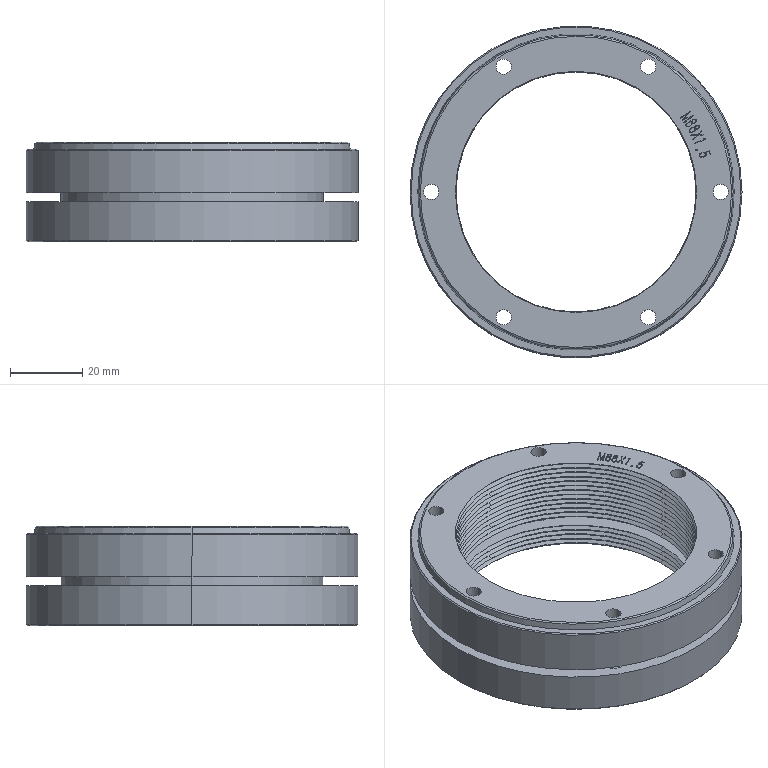Part | STEP file | Spindle Rear Nut | 1 solid | 308 faces | box 91.8 x 91.8 x 27.6 mm | volume 66941 mm3 | plane 89 | cone 88 | spline 67 | cylinder 64 | commonest cylinder face diameters 6.2 x16 4.2 x12 6.3 x12 9 x12 85.6 x6 91.8 x4